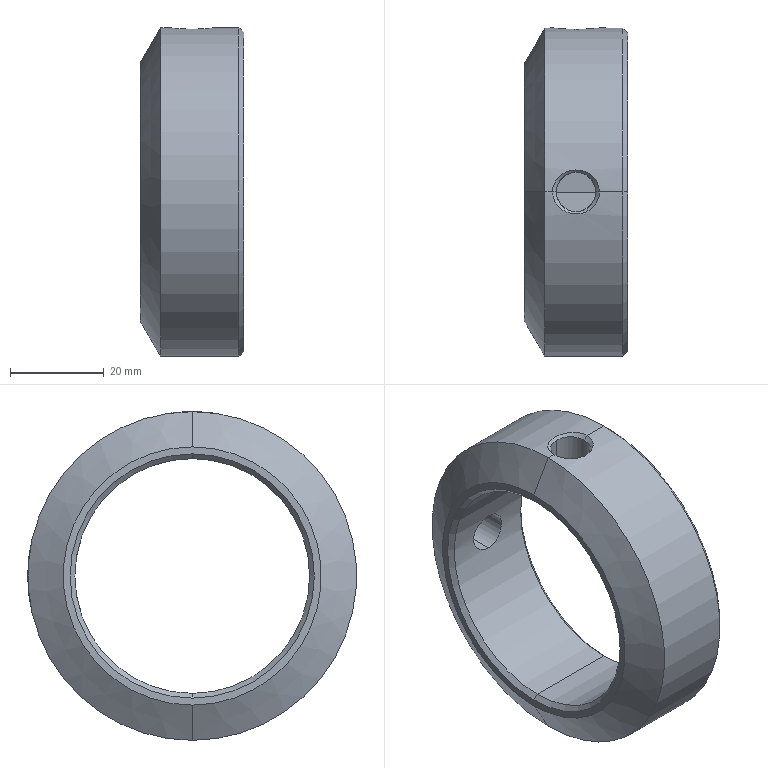Part | STEP file | 0229_Z_SCCN50-22_1 | 1 solid | 22 faces | box 22 x 70 x 70 mm | volume 36768 mm3 | cone 12 | cylinder 8 | plane 2 | commonest cylinder face diameters 8.376 x4 50 x2 70 x2